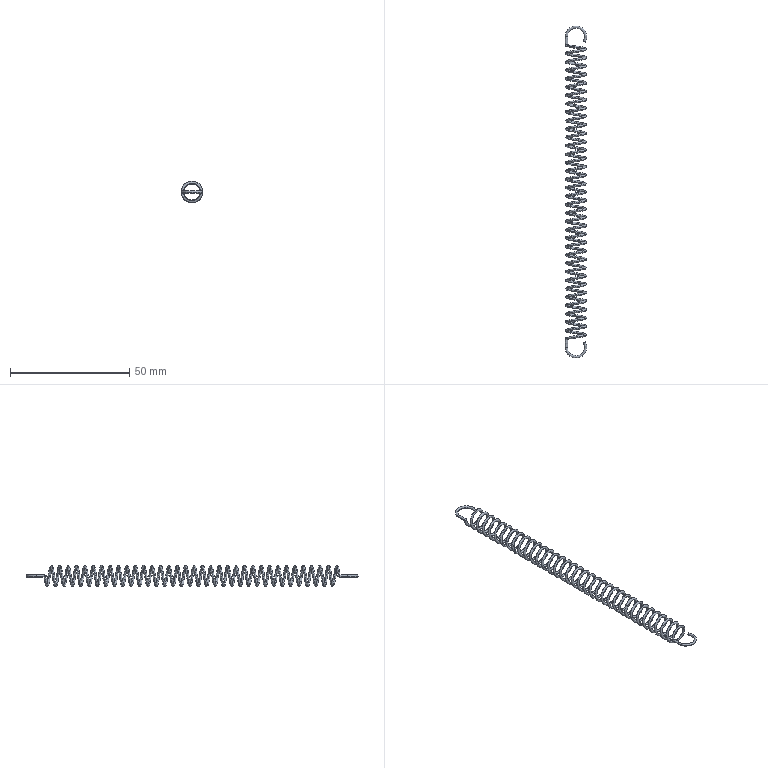Part | STEP file | 1 solid | 14 faces | box 9.014 x 139 x 9.007 mm | volume 726.563 mm3 | spline 12 | plane 2